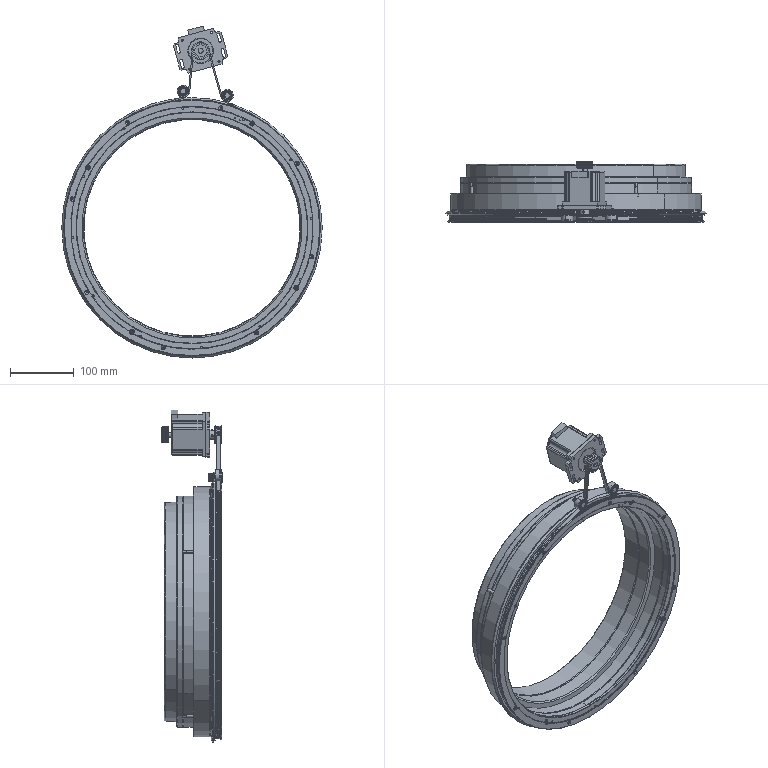Part | NX | features BREP 19 | 36 solids | 5924 faces | volume 1411287 mm3 | cylinder 4260 | plane 1193 | cone 413 | torus 38 | sphere 16 | spline 4 | commonest cylinder face diameters 0.5 x1022 3.04 x936 1.7 x579 396.69 x416 25 x371 6 x121